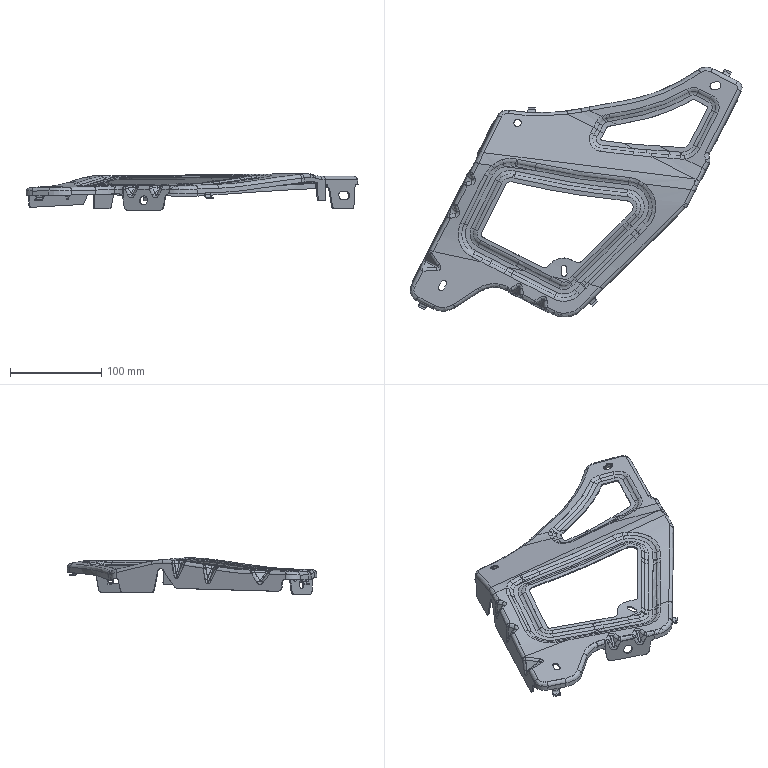Part | STEP file | Body.3_id638_x_t | 1 solid | 702 faces | box 364.651 x 274.568 x 40.313 mm | volume 69490 mm3 | spline 504 | cylinder 87 | plane 74 | sphere 20 | other 17 | commonest cylinder face diameters 5.5 x28 8 x22 3 x6 8.2 x5 6 x4 4 x3